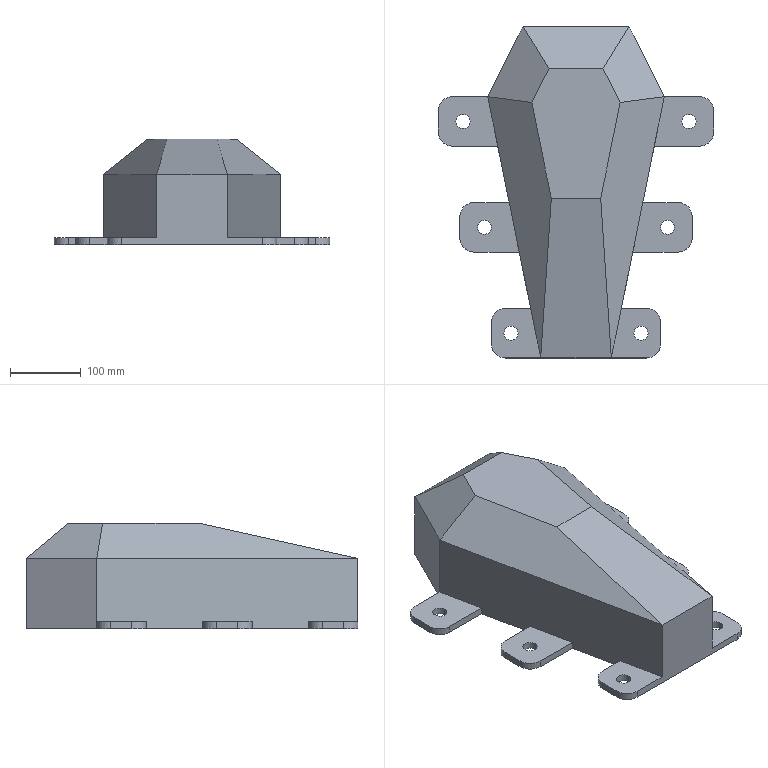Part | SolidWorks | features ICE 16, Fillet 3, Extrusion 1, MirrorPattern 1, Shell 1 | 1 solid | 74 faces | box 390 x 470 x 150 mm | volume 2183743 mm3 | plane 50 | cylinder 24 | commonest cylinder face diameters 20 x12 40 x12